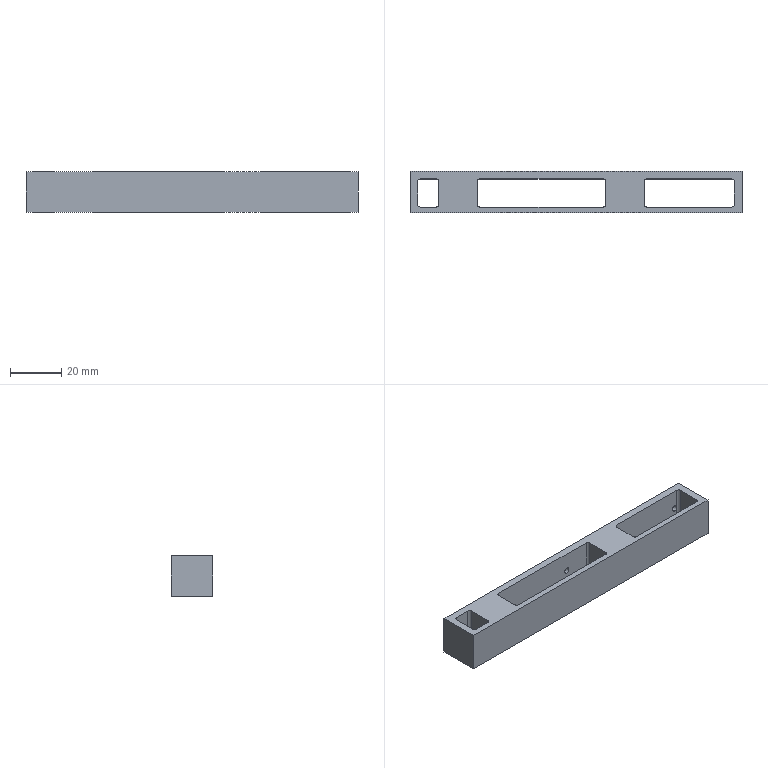NC program | NX | posted with a generic post | part box 130 x 16.2 x 16 mm
Lines 1 to 948 of 19599:
N10 G17 G21 G94 G90
(FLOOR_WALL , TOOL : D63)
N12 T01 M6
N14 G54
N16 G17 G0 G90 X-101.5 Y0. B0. C0. S6500 M3
N18 G43 Z30. H1
N20 Z3.
N22 G94 G1 Z0. F1250.
N24 X-98.5
N26 X98.5
N28 X101.5
N30 Z3.
N32 G0 Z30.
N34 M5
(ZLEVEL_PROFILE , TOOL : D10)
N36 T10 M6
N38 G54
N40 G17 G0 G90 X-49.567 Y-13.2 B0. C0. S9500 M3
N42 G43 Z30. H10
N44 Z1.5
N46 G94 G1 X-65. Z0.691 F1000.
N48 X-65.554 Z0.662
N50 X-66.898 Y-12.866 Z0.59
N52 X-68.104 Y-12.184 Z0.517
N54 X-69.084 Y-11.204 Z0.444
N56 X-69.766 Y-9.998 Z0.372
N58 X-70.1 Y-8.654 Z0.299
N60 Y-8.1 Z0.27
N62 Y8.1 Z-0.579
N64 Y8.654 Z-0.608
N66 X-69.766 Y9.998 Z-0.681
N68 X-69.084 Y11.204 Z-0.753
N70 X-68.104 Y12.184 Z-0.826
N72 X-66.898 Y12.866 Z-0.898
N74 X-65.554 Y13.2 Z-0.971
N76 X-65. Z-1.
N78 X65. F2500.
N80 G2 X70.1 Y8.1 R5.1
N82 G1 Y-8.1
N84 G2 X65. Y-13.2 R5.1
N86 G1 X-65.
N88 G2 X-70.1 Y-8.1 R5.1
N90 G1 Y8.1
N92 G2 X-65. Y13.2 R5.1
N94 G1 X-7.71 Z-2.
N96 X65.
N98 G2 X70.1 Y8.1 R5.1
N100 G1 Y-8.1
N102 G2 X65. Y-13.2 R5.1
N104 G1 X-65.
N106 G2 X-70.1 Y-8.1 R5.1
N108 G1 Y8.1
N110 G2 X-65. Y13.2 R5.1
N112 G1 X-7.71 Z-3.
N114 X65.
N116 G2 X70.1 Y8.1 R5.1
N118 G1 Y-8.1
N120 G2 X65. Y-13.2 R5.1
N122 G1 X-65.
N124 G2 X-70.1 Y-8.1 R5.1
N126 G1 Y8.1
N128 G2 X-65. Y13.2 R5.1
N130 G1 X-7.71 Z-4.
N132 X65.
N134 G2 X70.1 Y8.1 R5.1
N136 G1 Y-8.1
N138 G2 X65. Y-13.2 R5.1
N140 G1 X-65.
N142 G2 X-70.1 Y-8.1 R5.1
N144 G1 Y8.1
N146 G2 X-65. Y13.2 R5.1
N148 G1 X-7.71 Z-5.
N150 X65.
N152 G2 X70.1 Y8.1 R5.1
N154 G1 Y-8.1
N156 G2 X65. Y-13.2 R5.1
N158 G1 X-65.
N160 G2 X-70.1 Y-8.1 R5.1
N162 G1 Y8.1
N164 G2 X-65. Y13.2 R5.1
N166 G1 X-7.71 Z-6.
N168 X65.
N170 G2 X70.1 Y8.1 R5.1
N172 G1 Y-8.1
N174 G2 X65. Y-13.2 R5.1
N176 G1 X-65.
N178 G2 X-70.1 Y-8.1 R5.1
N180 G1 Y8.1
N182 G2 X-65. Y13.2 R5.1
N184 G1 X-7.71 Z-7.
N186 X65.
N188 G2 X70.1 Y8.1 R5.1
N190 G1 Y-8.1
N192 G2 X65. Y-13.2 R5.1
N194 G1 X-65.
N196 G2 X-70.1 Y-8.1 R5.1
N198 G1 Y8.1
N200 G2 X-65. Y13.2 R5.1
N202 G1 X-7.71 Z-8.
N204 X65.
N206 G2 X70.1 Y8.1 R5.1
N208 G1 Y-8.1
N210 G2 X65. Y-13.2 R5.1
N212 G1 X-65.
N214 G2 X-70.1 Y-8.1 R5.1
N216 G1 Y8.1
N218 G2 X-65. Y13.2 R5.1
N220 G1 X-7.71 Z-9.
N222 X65.
N224 G2 X70.1 Y8.1 R5.1
N226 G1 Y-8.1
N228 G2 X65. Y-13.2 R5.1
N230 G1 X-65.
N232 G2 X-70.1 Y-8.1 R5.1
N234 G1 Y8.1
N236 G2 X-65. Y13.2 R5.1
N238 G1 X-7.71 Z-10.
N240 X65.
N242 G2 X70.1 Y8.1 R5.1
N244 G1 Y-8.1
N246 G2 X65. Y-13.2 R5.1
N248 G1 X-65.
N250 G2 X-70.1 Y-8.1 R5.1
N252 G1 Y8.1
N254 G2 X-65. Y13.2 R5.1
N256 G1 X-7.71 Z-11.
N258 X65.
N260 G2 X70.1 Y8.1 R5.1
N262 G1 Y-8.1
N264 G2 X65. Y-13.2 R5.1
N266 G1 X-65.
N268 G2 X-70.1 Y-8.1 R5.1
N270 G1 Y8.1
N272 G2 X-65. Y13.2 R5.1
N274 G1 X-7.71 Z-12.
N276 X65.
N278 G2 X70.1 Y8.1 R5.1
N280 G1 Y-8.1
N282 G2 X65. Y-13.2 R5.1
N284 G1 X-65.
N286 G2 X-70.1 Y-8.1 R5.1
N288 G1 Y8.1
N290 G2 X-65. Y13.2 R5.1
N292 G1 X-7.71 Z-13.
N294 X65.
N296 G2 X70.1 Y8.1 R5.1
N298 G1 Y-8.1
N300 G2 X65. Y-13.2 R5.1
N302 G1 X-65.
N304 G2 X-70.1 Y-8.1 R5.1
N306 G1 Y8.1
N308 G2 X-65. Y13.2 R5.1
N310 G1 X-7.71 Z-14.
N312 X65.
N314 G2 X70.1 Y8.1 R5.1
N316 G1 Y-8.1
N318 G2 X65. Y-13.2 R5.1
N320 G1 X-65.
N322 G2 X-70.1 Y-8.1 R5.1
N324 G1 Y8.1
N326 G2 X-65. Y13.2 R5.1
N328 G1 X-7.71 Z-15.
N330 X65.
N332 G2 X70.1 Y8.1 R5.1
N334 G1 Y-8.1
N336 G2 X65. Y-13.2 R5.1
N338 G1 X-65.
N340 G2 X-70.1 Y-8.1 R5.1
N342 G1 Y8.1
N344 G2 X-65. Y13.2 R5.1
N346 G1 X-7.71 Z-16.
N348 X65.
N350 G2 X70.1 Y8.1 R5.1
N352 G1 Y-8.1
N354 G2 X65. Y-13.2 R5.1
N356 G1 X-65.
N358 G2 X-70.1 Y-8.1 R5.1
N360 G1 Y8.1
N362 G2 X-65. Y13.2 R5.1
N364 G1 X-7.71
N366 Z-14.5
N368 G0 Z30.
(ZLEVEL_PROFILE_COPY , TOOL : D10)
N370 X-66.622 Y14.909
N372 Z-14.5
N374 G1 Z-16. F1000.
N376 X-65.866 Y13.6
N378 G3 X-65. Y13.1 R1.
N380 G1 X65. F1200.
N382 G2 X70. Y8.1 R5.
N384 G1 Y-8.1
N386 G2 X65. Y-13.1 R5.
N388 G1 X-65.
N390 G2 X-70. Y-8.1 R5.
N392 G1 Y8.1
N394 G2 X-65. Y13.1 R5.
N396 G3 X-64.134 Y13.6 R1.
N398 G1 X-63.268 Y15.1
N400 Z-14.5
N402 G0 Z30.
N404 M5
(ZLEVEL_PROFILE_COPY_1 , TOOL : D6)
N406 T06 M6
N408 G54
N410 G17 G0 G90 X58.9 Y-1.975 B0. C0. S9500 M3
N412 G43 Z30. H6
N414 Z1.5
N416 G94 G1 Y2. Z1.292 F1000.
N418 X29.802 Z-0.233
N420 Y-2.8 Z-0.485
N422 X58.9 F2500.
N424 Y2.
N426 X29.802
N428 Y-2.8
N430 X57.579 Z-0.97
N432 X58.9
N434 Y2.
N436 X29.802
N438 Y-2.8
N440 X57.579 Z-1.455
N442 X58.9
N444 Y2.
N446 X29.802
N448 Y-2.8
N450 X57.579 Z-1.939
N452 X58.9
N454 Y2.
N456 X29.802
N458 Y-2.8
N460 X57.579 Z-2.424
N462 X58.9
N464 Y2.
N466 X29.802
N468 Y-2.8
N470 X57.579 Z-2.909
N472 X58.9
N474 Y2.
N476 X29.802
N478 Y-2.8
N480 X57.579 Z-3.394
N482 X58.9
N484 Y2.
N486 X29.802
N488 Y-2.8
N490 X57.579 Z-3.879
N492 X58.9
N494 Y2.
N496 X29.802
N498 Y-2.8
N500 X57.579 Z-4.364
N502 X58.9
N504 Y2.
N506 X29.802
N508 Y-2.8
N510 X57.579 Z-4.848
N512 X58.9
N514 Y2.
N516 X29.802
N518 Y-2.8
N520 X57.579 Z-5.333
N522 X58.9
N524 Y2.
N526 X29.802
N528 Y-2.8
N530 X57.579 Z-5.818
N532 X58.9
N534 Y2.
N536 X29.802
N538 Y-2.8
N540 X57.579 Z-6.303
N542 X58.9
N544 Y2.
N546 X29.802
N548 Y-2.8
N550 X57.579 Z-6.788
N552 X58.9
N554 Y2.
N556 X29.802
N558 Y-2.8
N560 X57.579 Z-7.273
N562 X58.9
N564 Y2.
N566 X29.802
N568 Y-2.8
N570 X57.579 Z-7.758
N572 X58.9
N574 Y2.
N576 X29.802
N578 Y-2.8
N580 X57.579 Z-8.242
N582 X58.9
N584 Y2.
N586 X29.802
N588 Y-2.8
N590 X57.579 Z-8.727
N592 X58.9
N594 Y2.
N596 X29.802
N598 Y-2.8
N600 X57.579 Z-9.212
N602 X58.9
N604 Y2.
N606 X29.802
N608 Y-2.8
N610 X57.579 Z-9.697
N612 X58.9
N614 Y2.
N616 X29.802
N618 Y-2.8
N620 X57.579 Z-10.182
N622 X58.9
N624 Y2.
N626 X29.802
N628 Y-2.8
N630 X57.579 Z-10.667
N632 X58.9
N634 Y2.
N636 X29.802
N638 Y-2.8
N640 X57.579 Z-11.152
N642 X58.9
N644 Y2.
N646 X29.802
N648 Y-2.8
N650 X57.579 Z-11.636
N652 X58.9
N654 Y2.
N656 X29.802
N658 Y-2.8
N660 X57.579 Z-12.121
N662 X58.9
N664 Y2.
N666 X29.802
N668 Y-2.8
N670 X57.579 Z-12.606
N672 X58.9
N674 Y2.
N676 X29.802
N678 Y-2.8
N680 X57.579 Z-13.091
N682 X58.9
N684 Y2.
N686 X29.802
N688 Y-2.8
N690 X57.579 Z-13.576
N692 X58.9
N694 Y2.
N696 X29.802
N698 Y-2.8
N700 X57.579 Z-14.061
N702 X58.9
N704 Y2.
N706 X29.802
N708 Y-2.8
N710 X57.579 Z-14.545
N712 X58.9
N714 Y2.
N716 X29.802
N718 Y-2.8
N720 X57.579 Z-15.03
N722 X58.9
N724 Y2.
N726 X29.802
N728 Y-2.8
N730 X57.579 Z-15.515
N732 X58.9
N734 Y2.
N736 X29.802
N738 Y-2.8
N740 X57.579 Z-16.
N742 X58.9
N744 Y2.
N746 X29.802
N748 Y-2.8
N750 X57.579
N752 Z-14.5
N754 G0 Z30.
N756 X-2.535 Y2.
N758 Z1.5
N760 G1 X-35.608 Z-0.233 F1000.
N762 Y-2.8 Z-0.485
N764 X8.602 F2500.
N766 Y2.
N768 X-35.608
N770 Y-2.8
N772 X-7.831 Z-0.97
N774 X8.602
N776 Y2.
N778 X-35.608
N780 Y-2.8
N782 X-7.831 Z-1.455
N784 X8.602
N786 Y2.
N788 X-35.608
N790 Y-2.8
N792 X-7.831 Z-1.939
N794 X8.602
N796 Y2.
N798 X-35.608
N800 Y-2.8
N802 X-7.831 Z-2.424
N804 X8.602
N806 Y2.
N808 X-35.608
N810 Y-2.8
N812 X-7.831 Z-2.909
N814 X8.602
N816 Y2.
N818 X-35.608
N820 Y-2.8
N822 X-7.831 Z-3.394
N824 X8.602
N826 Y2.
N828 X-35.608
N830 Y-2.8
N832 X-7.831 Z-3.879
N834 X8.602
N836 Y2.
N838 X-35.608
N840 Y-2.8
N842 X-7.831 Z-4.364
N844 X8.602
N846 Y2.
N848 X-35.608
N850 Y-2.8
N852 X-7.831 Z-4.848
N854 X8.602
N856 Y2.
N858 X-35.608
N860 Y-2.8
N862 X-7.831 Z-5.333
N864 X8.602
N866 Y2.
N868 X-35.608
N870 Y-2.8
N872 X-7.831 Z-5.818
N874 X8.602
N876 Y2.
N878 X-35.608
N880 Y-2.8
N882 X-7.831 Z-6.303
N884 X8.602
N886 Y2.
N888 X-35.608
N890 Y-2.8
N892 X-7.831 Z-6.788
N894 X8.602
N896 Y2.
N898 X-35.608
N900 Y-2.8
N902 X-7.831 Z-7.273
N904 X8.602
N906 Y2.
N908 X-35.608
N910 Y-2.8
N912 X-7.831 Z-7.758
N914 X8.602
N916 Y2.
N918 X-35.608
N920 Y-2.8
N922 X-7.831 Z-8.242
N924 X8.602
N926 Y2.
N928 X-35.608
N930 Y-2.8
N932 X-7.831 Z-8.727
N934 X8.602
N936 Y2.
N938 X-35.608
N940 Y-2.8
N942 X-7.831 Z-9.212
N944 X8.602
N946 Y2.
N948 X-35.608
N950 Y-2.8
N952 X-7.831 Z-9.697
N954 X8.602
N956 Y2.
N958 X-35.608
N960 Y-2.8
N962 X-7.831 Z-10.182
N964 X8.602
N966 Y2.
N968 X-35.608
N970 Y-2.8
N972 X-7.831 Z-10.667
N974 X8.602
N976 Y2.
N978 X-35.608
N980 Y-2.8
N982 X-7.831 Z-11.152
N984 X8.602
N986 Y2.
N988 X-35.608
N990 Y-2.8
N992 X-7.831 Z-11.636
N994 X8.602
N996 Y2.
N998 X-35.608
N1000 Y-2.8
N1002 X-7.831 Z-12.121
N1004 X8.602
N1006 Y2.
N1008 X-35.608
N1010 Y-2.8
N1012 X-7.831 Z-12.606
N1014 X8.602
N1016 Y2.
N1018 X-35.608
N1020 Y-2.8
N1022 X-7.831 Z-13.091
N1024 X8.602
N1026 Y2.
N1028 X-35.608
N1030 Y-2.8
N1032 X-7.831 Z-13.576
N1034 X8.602
N1036 Y2.
N1038 X-35.608
N1040 Y-2.8
N1042 X-7.831 Z-14.061
N1044 X8.602
N1046 Y2.
N1048 X-35.608
N1050 Y-2.8
N1052 X-7.831 Z-14.545
N1054 X8.602
N1056 Y2.
N1058 X-35.608
N1060 Y-2.8
N1062 X-7.831 Z-15.03
N1064 X8.602
N1066 Y2.
N1068 X-35.608
N1070 Y-2.8
N1072 X-7.831 Z-15.515
N1074 X8.602
N1076 Y2.
N1078 X-35.608
N1080 Y-2.8
N1082 X-7.831 Z-16.
N1084 X8.602
N1086 Y2.
N1088 X-35.608
N1090 Y-2.8
N1092 X-7.831
N1094 Z-14.5
N1096 G0 Z30.
N1098 X-58.9 Y-1.478
N1100 Z1.5
N1102 G1 Y-2.8 Z1.431 F1000.
N1104 X-56.808 Z1.321
N1106 Y2. Z1.07
N1108 X-58.9 Z0.96
N1110 Y-2.8 Z0.708
N1112 X-56.808 Z0.599
N1114 Y2. Z0.347
N1116 X-58.9 Z0.238
N1118 Y-2.8 Z-0.014
N1120 X-56.808 Z-0.124
N1122 Y2. Z-0.375
N1124 X-58.9 Z-0.485
N1126 Y-2.8 F2500.
N1128 X-56.808
N1130 Y2.
N1132 X-58.9
N1134 Y-2.726 Z-0.706
N1136 X-58.679 Y-2.8 Z-0.72
N1138 X-56.907 Z-0.803
N1140 X-56.808 Y-2.603 Z-0.817
N1142 Y0.646 Z-0.97
N1144 Y2.
N1146 X-58.9
N1148 Y-2.726 Z-1.191
N1150 X-58.679 Y-2.8 Z-1.205
N1152 X-56.907 Z-1.288
N1154 X-56.808 Y-2.603 Z-1.302
N1156 Y0.646 Z-1.455
N1158 Y2.
N1160 X-58.9
N1162 Y-2.726 Z-1.676
N1164 X-58.679 Y-2.8 Z-1.69
N1166 X-56.907 Z-1.773
N1168 X-56.808 Y-2.603 Z-1.787
N1170 Y0.646 Z-1.939
N1172 Y2.
N1174 X-58.9
N1176 Y-2.726 Z-2.161
N1178 X-58.679 Y-2.8 Z-2.175
N1180 X-56.907 Z-2.258
N1182 X-56.808 Y-2.603 Z-2.272
N1184 Y0.646 Z-2.424
N1186 Y2.
N1188 X-58.9
N1190 Y-2.726 Z-2.646
N1192 X-58.679 Y-2.8 Z-2.66
N1194 X-56.907 Z-2.743
N1196 X-56.808 Y-2.603 Z-2.757
N1198 Y0.646 Z-2.909
N1200 Y2.
N1202 X-58.9
N1204 Y-2.726 Z-3.131
N1206 X-58.679 Y-2.8 Z-3.145
N1208 X-56.907 Z-3.228
N1210 X-56.808 Y-2.603 Z-3.242
N1212 Y0.646 Z-3.394
N1214 Y2.
N1216 X-58.9
N1218 Y-2.726 Z-3.616
N1220 X-58.679 Y-2.8 Z-3.629
N1222 X-56.907 Z-3.713
N1224 X-56.808 Y-2.603 Z-3.726
N1226 Y0.646 Z-3.879
N1228 Y2.
N1230 X-58.9
N1232 Y-2.726 Z-4.1
N1234 X-58.679 Y-2.8 Z-4.114
N1236 X-56.907 Z-4.197
N1238 X-56.808 Y-2.603 Z-4.211
N1240 Y0.646 Z-4.364
N1242 Y2.
N1244 X-58.9
N1246 Y-2.726 Z-4.585
N1248 X-58.679 Y-2.8 Z-4.599
N1250 X-56.907 Z-4.682
N1252 X-56.808 Y-2.603 Z-4.696
N1254 Y0.646 Z-4.848
N1256 Y2.
N1258 X-58.9
N1260 Y-2.726 Z-5.07
N1262 X-58.679 Y-2.8 Z-5.084
N1264 X-56.907 Z-5.167
N1266 X-56.808 Y-2.603 Z-5.181
N1268 Y0.646 Z-5.333
N1270 Y2.
N1272 X-58.9
N1274 Y-2.726 Z-5.555
N1276 X-58.679 Y-2.8 Z-5.569
N1278 X-56.907 Z-5.652
N1280 X-56.808 Y-2.603 Z-5.666
N1282 Y0.646 Z-5.818
N1284 Y2.
N1286 X-58.9
N1288 Y-2.726 Z-6.04
N1290 X-58.679 Y-2.8 Z-6.054
N1292 X-56.907 Z-6.137
N1294 X-56.808 Y-2.603 Z-6.151
N1296 Y0.646 Z-6.303
N1298 Y2.
N1300 X-58.9
N1302 Y-2.726 Z-6.525
N1304 X-58.679 Y-2.8 Z-6.539
N1306 X-56.907 Z-6.622
N1308 X-56.808 Y-2.603 Z-6.635
N1310 Y0.646 Z-6.788
N1312 Y2.
N1314 X-58.9
N1316 Y-2.726 Z-7.01
N1318 X-58.679 Y-2.8 Z-7.023
N1320 X-56.907 Z-7.106
N1322 X-56.808 Y-2.603 Z-7.12
N1324 Y0.646 Z-7.273
N1326 Y2.
N1328 X-58.9
N1330 Y-2.726 Z-7.494
N1332 X-58.679 Y-2.8 Z-7.508
N1334 X-56.907 Z-7.591
N1336 X-56.808 Y-2.603 Z-7.605
N1338 Y0.646 Z-7.758
N1340 Y2.
N1342 X-58.9
N1344 Y-2.726 Z-7.979
N1346 X-58.679 Y-2.8 Z-7.993
N1348 X-56.907 Z-8.076
N1350 X-56.808 Y-2.603 Z-8.09
N1352 Y0.646 Z-8.242
N1354 Y2.
N1356 X-58.9
N1358 Y-2.726 Z-8.464
N1360 X-58.679 Y-2.8 Z-8.478
N1362 X-56.907 Z-8.561
N1364 X-56.808 Y-2.603 Z-8.575
N1366 Y0.646 Z-8.727
N1368 Y2.
N1370 X-58.9
N1372 Y-2.726 Z-8.949
N1374 X-58.679 Y-2.8 Z-8.963
N1376 X-56.907 Z-9.046
N1378 X-56.808 Y-2.603 Z-9.06
N1380 Y0.646 Z-9.212
N1382 Y2.
N1384 X-58.9
N1386 Y-2.726 Z-9.434
N1388 X-58.679 Y-2.8 Z-9.448
N1390 X-56.907 Z-9.531
N1392 X-56.808 Y-2.603 Z-9.545
N1394 Y0.646 Z-9.697
N1396 Y2.
N1398 X-58.9
N1400 Y-2.726 Z-9.919
N1402 X-58.679 Y-2.8 Z-9.932
N1404 X-56.907 Z-10.016
N1406 X-56.808 Y-2.603 Z-10.029
N1408 Y0.646 Z-10.182
N1410 Y2.
N1412 X-58.9
N1414 Y-2.726 Z-10.403
N1416 X-58.679 Y-2.8 Z-10.417
N1418 X-56.907 Z-10.5
N1420 X-56.808 Y-2.603 Z-10.514
N1422 Y0.646 Z-10.667
N1424 Y2.
N1426 X-58.9
N1428 Y-2.726 Z-10.888
N1430 X-58.679 Y-2.8 Z-10.902
N1432 X-56.907 Z-10.985
N1434 X-56.808 Y-2.603 Z-10.999
N1436 Y0.646 Z-11.152
N1438 Y2.
N1440 X-58.9
N1442 Y-2.726 Z-11.373
N1444 X-58.679 Y-2.8 Z-11.387
N1446 X-56.907 Z-11.47
N1448 X-56.808 Y-2.603 Z-11.484
N1450 Y0.646 Z-11.636
N1452 Y2.
N1454 X-58.9
N1456 Y-2.726 Z-11.858
N1458 X-58.679 Y-2.8 Z-11.872
N1460 X-56.907 Z-11.955
N1462 X-56.808 Y-2.603 Z-11.969
N1464 Y0.646 Z-12.121
N1466 Y2.
N1468 X-58.9
N1470 Y-2.726 Z-12.343
N1472 X-58.679 Y-2.8 Z-12.357
N1474 X-56.907 Z-12.44
N1476 X-56.808 Y-2.603 Z-12.454
N1478 Y0.646 Z-12.606
N1480 Y2.
N1482 X-58.9
N1484 Y-2.726 Z-12.828
N1486 X-58.679 Y-2.8 Z-12.842
N1488 X-56.907 Z-12.925
N1490 X-56.808 Y-2.603 Z-12.939
N1492 Y0.646 Z-13.091
N1494 Y2.
N1496 X-58.9
N1498 Y-2.726 Z-13.313
N1500 X-58.679 Y-2.8 Z-13.326
N1502 X-56.907 Z-13.41
N1504 X-56.808 Y-2.603 Z-13.423
N1506 Y0.646 Z-13.576
N1508 Y2.
N1510 X-58.9
N1512 Y-2.726 Z-13.797
N1514 X-58.679 Y-2.8 Z-13.811
N1516 X-56.907 Z-13.894
N1518 X-56.808 Y-2.603 Z-13.908
N1520 Y0.646 Z-14.061
N1522 Y2.
N1524 X-58.9
N1526 Y-2.726 Z-14.282
N1528 X-58.679 Y-2.8 Z-14.296
N1530 X-56.907 Z-14.379
N1532 X-56.808 Y-2.603 Z-14.393
N1534 Y0.646 Z-14.545
N1536 Y2.
N1538 X-58.9
N1540 Y-2.726 Z-14.767
N1542 X-58.679 Y-2.8 Z-14.781
N1544 X-56.907 Z-14.864
N1546 X-56.808 Y-2.603 Z-14.878
N1548 Y0.646 Z-15.03
N1550 Y2.
N1552 X-58.9
N1554 Y-2.726 Z-15.252
N1556 X-58.679 Y-2.8 Z-15.266
N1558 X-56.907 Z-15.349
N1560 X-56.808 Y-2.603 Z-15.363
N1562 Y0.646 Z-15.515
N1564 Y2.
N1566 X-58.9
N1568 Y-2.726 Z-15.737
N1570 X-58.679 Y-2.8 Z-15.751
N1572 X-56.907 Z-15.834
N1574 X-56.808 Y-2.603 Z-15.848
N1576 Y0.646 Z-16.
N1578 Y2.
N1580 X-58.9
N1582 Y-2.8
N1584 X-56.808
N1586 Y0.646
N1588 Z-14.5
N1590 G0 Z30.
(ZLEVEL_PROFILE_COPY_COPY , TOOL : D6)
N1592 X-34.582 Y2.1
N1594 Z1.5
N1596 G1 X-35.708 Z1.441 F1000.
N1598 Y-2.9 Z1.179
N1600 X8.702 Z-1.148
N1602 Y2.1 Z-1.411
N1604 X-35.708 Z-3.738
N1606 Y-2.9 Z-4.
N1608 X8.702 F1200.
N1610 Y2.1
N1612 X-35.708
N1614 Y-2.9
N1616 X8.522 Z-6.387
N1618 X8.702 Y-2.781 Z-6.403
N1620 Y2. Z-6.661
N1622 X8.503 Y2.1 Z-6.677
N1624 X-16.003 Z-8.
N1626 X-35.708
N1628 Y-2.9
N1630 X8.522 Z-10.387
N1632 X8.702 Y-2.781 Z-10.403
N1634 Y2. Z-10.661
N1636 X8.503 Y2.1 Z-10.677
N1638 X-16.003 Z-12.
N1640 X-35.708
N1642 Y-2.9
N1644 X8.522 Z-14.387
N1646 X8.702 Y-2.781 Z-14.403
N1648 Y2. Z-14.661
N1650 X8.503 Y2.1 Z-14.677
N1652 X-16.003 Z-16.
N1654 X-35.708
N1656 Y-2.9
N1658 X8.702
N1660 Y2.1
N1662 X-16.003
N1664 Z-14.5
N1666 G0 Z30.
N1668 X59. Y0.048
N1670 Z1.5
N1672 G1 Y2.1 Z1.392 F1000.
N1674 X29.702 Z-0.143
N1676 Y-2.9 Z-0.405
N1678 X59. Z-1.94
N1680 Y2.1 Z-2.203
N1682 X29.702 Z-3.738
N1684 Y-2.9 Z-4.
N1686 X59. F1200.
N1688 Y2.1
N1690 X29.702
N1692 Y-2.9
N1694 X58.716 Z-6.256
N1696 X59. Y-2.885 Z-6.279
N1698 Y1.901 Z-6.651
N1700 X58.9 Y2.1 Z-6.674
N1702 X41.851 Z-8.
N1704 X29.702
N1706 Y-2.9
N1708 X58.716 Z-10.256
N1710 X59. Y-2.885 Z-10.279
N1712 Y1.901 Z-10.651
N1714 X58.9 Y2.1 Z-10.674
N1716 X41.851 Z-12.
N1718 X29.702
N1720 Y-2.9
N1722 X58.716 Z-14.256
N1724 X59. Y-2.885 Z-14.279
N1726 Y1.901 Z-14.651
N1728 X58.9 Y2.1 Z-14.674
N1730 X41.851 Z-16.
N1732 X29.702
N1734 Y-2.9
N1736 X59.
N1738 Y2.1
N1740 X41.851
N1742 Z-14.5
N1744 G0 Z30.
N1746 X-56.708 Y1.532
N1748 Z1.5
N1750 G1 Y2.1 Z1.47 F1000.
N1752 X-59. Z1.35
N1754 Y-2.9 Z1.088
N1756 X-56.708 Z0.968
N1758 Y2.1 Z0.706
N1760 X-59. Z0.586
N1762 Y-2.9 Z0.324
N1764 X-56.708 Z0.204
N1766 Y2.1 Z-0.058
N1768 X-59. Z-0.178
N1770 Y-2.9 Z-0.441
N1772 X-56.708 Z-0.561
N1774 Y2.1 Z-0.823
N1776 X-59. Z-0.943
N1778 Y-2.9 Z-1.205
N1780 X-56.708 Z-1.325
N1782 Y2.1 Z-1.587
N1784 X-59. Z-1.707
N1786 Y-2.9 Z-1.969
N1788 X-56.708 Z-2.089
N1790 Y2.1 Z-2.351
N1792 X-59. Z-2.471
N1794 Y-2.9 Z-2.733
N1796 X-56.708 Z-2.854
N1798 Y2.1 Z-3.116
N1800 X-59. Z-3.236
N1802 Y-2.9 Z-3.498
N1804 X-56.708 Z-3.618
N1806 Y2.1 Z-3.88
N1808 X-59. Z-4.
N1810 Y-2.9 F1200.
N1812 X-56.708
N1814 Y2.1
N1816 X-59.
N1818 Y-2.63 Z-5.73
N1820 X-58.975 Y-2.9 Z-5.838
N1822 X-56.905 Z-6.595
N1824 X-56.708 Y-2.801 Z-6.703
N1826 Y0.746 Z-8.
N1828 Y2.1
N1830 X-59.
N1832 Y-2.63 Z-9.73
N1834 X-58.975 Y-2.9 Z-9.838
N1836 X-56.905 Z-10.595
N1838 X-56.708 Y-2.801 Z-10.703
N1840 Y0.746 Z-12.
N1842 Y2.1
N1844 X-59.
N1846 Y-2.63 Z-13.73
N1848 X-58.975 Y-2.9 Z-13.838
N1850 X-56.905 Z-14.595
N1852 X-56.708 Y-2.801 Z-14.703
N1854 Y0.746 Z-16.
N1856 Y2.1
N1858 X-59.
N1860 Y-2.9
N1862 X-56.708
N1864 Y0.746
N1866 Z-14.5
N1868 G0 Z30.
N1870 M5